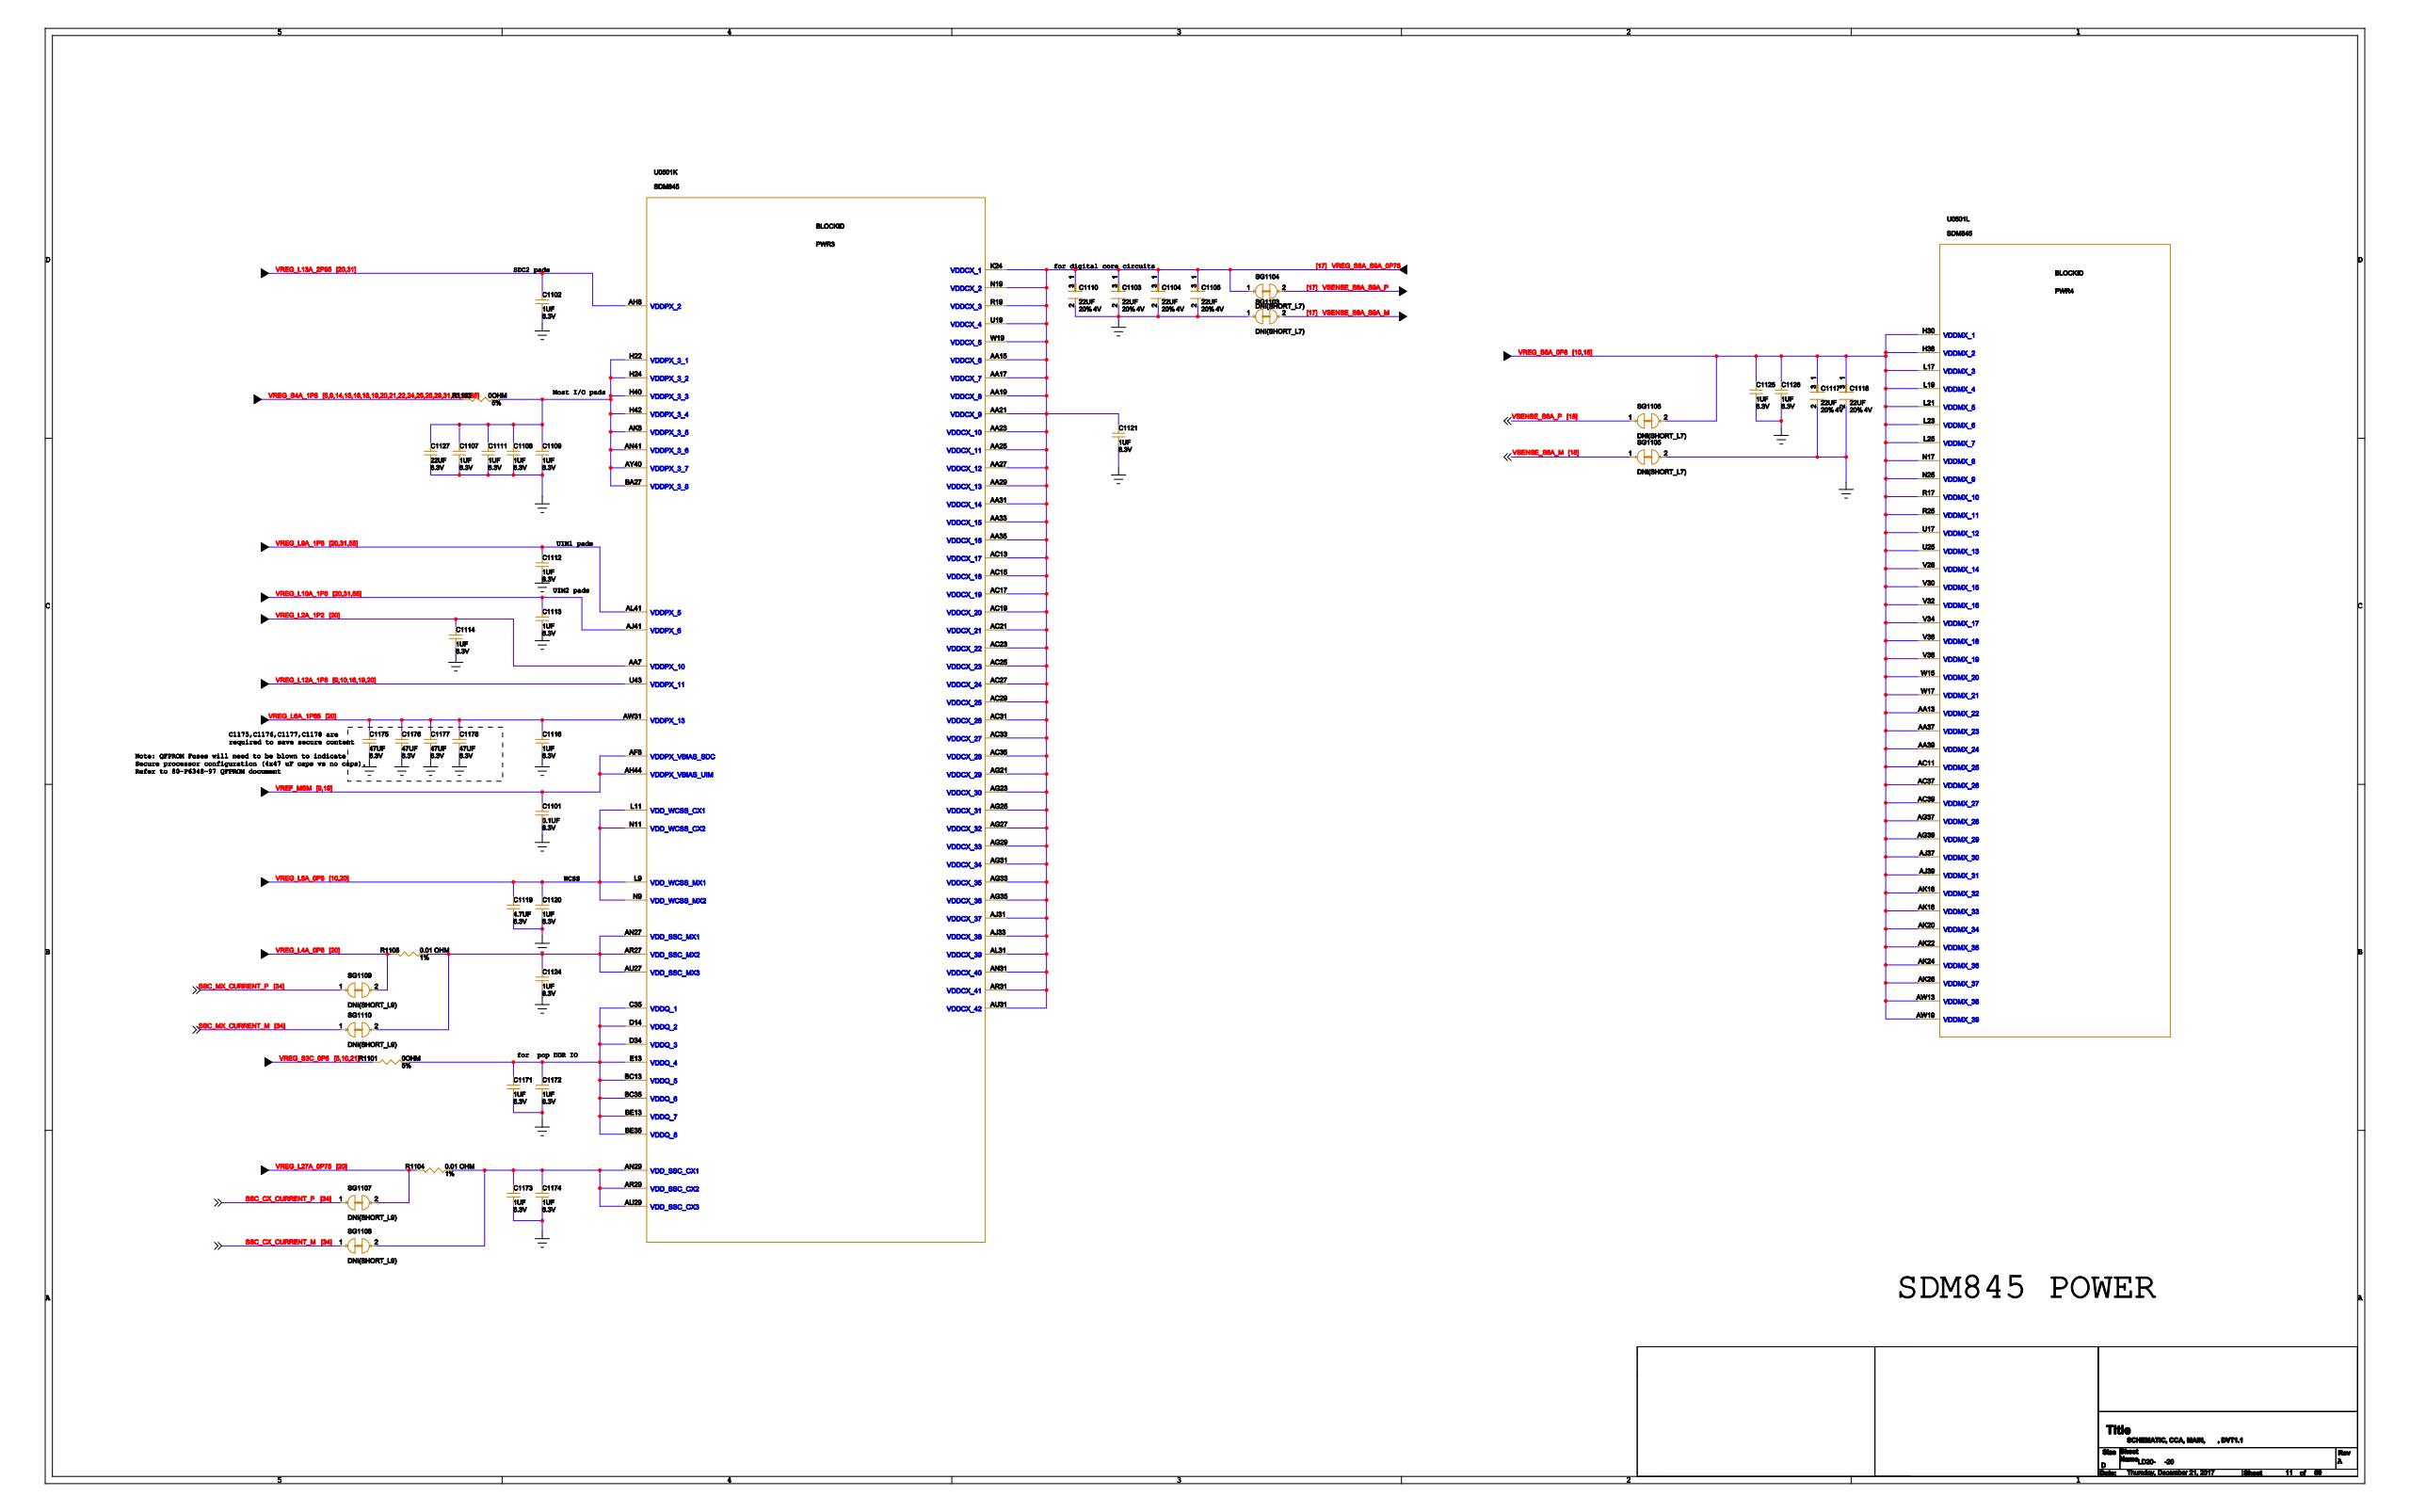Circuit board | Cadence Allegro | 1520 parts | 1149 nets | one sheet of the schematic
Parts on this sheet (reference | value | footprint):
C1101 | 0.1UF | 2P0201R
C1102 | 1UF | 2P0201R
C1103 | 22UF | 3PSM49X37N
C1104 | 22UF | 3PSM49X37N
C1105 | 22UF | 3PSM49X37N
C1107 | 1UF | 2P0201R
C1108 | 1UF | 2P0201R
C1109 | 1UF | 2P0201R
C1110 | 22UF | 3PSM49X37N
C1111 | 1UF | 2P0201R
C1112 | 1UF | 2P0201R
C1113 | 1UF | 2P0201R
C1114 | 1UF | 2P0201R
C1116 | 1UF | 2P0201R
C1117 | 22UF | 3PSM49X37N
C1118 | 22UF | 3PSM49X37N
C1119 | 4.7UF | 2P0402R
C1120 | 1UF | 2P0201R
C1121 | 1UF | 2P0201R
C1124 | 1UF | 2P0201R
C1125 | 1UF | 2P0201R
C1126 | 1UF | 2P0201R
C1127 | 22UF | 2P0603R
C1171 | 1UF | 2P0201R
C1172 | 1UF | 2P0201R
C1173 | 1UF | 2P0201R
C1174 | 1UF | 2P0201R
C1175 | 47UF | 2P0603R
C1176 | 47UF | 2P0603R
C1177 | 47UF | 2P0603R
C1178 | 47UF | 2P0603R
R1101 | 0OHM | 2P0201R
R1103 | 0OHM | 2P0201R
R1104 | 0.01 OHM | 2P0603R
R1105 | 0.01 OHM | 2P0603R
SG1103 | DNI(SHORT_L7) | SHORT_L7_2REC08X12
SG1104 | DNI(SHORT_L7) | SHORT_L7_2REC08X12
SG1105 | DNI(SHORT_L7) | SHORT_L7_2REC08X12
SG1106 | DNI(SHORT_L7) | SHORT_L7_2REC08X12
SG1107 | DNI(SHORT_L9) | SHORT_L9_2REC08X12
SG1108 | DNI(SHORT_L9) | SHORT_L9_2REC08X12
SG1109 | DNI(SHORT_L9) | SHORT_L9_2REC08X12
SG1110 | DNI(SHORT_L9) | SHORT_L9_2REC08X12
U0501 | SDM845 | 914PGA490X490B138D45
Nets of these parts (net: part-pin ...):
GND: C1101-2 C1102-2 C1103-2 C1104-2 C1105-2 C1107-2 C1108-2 C1109-2 C1110-2 C1111-2 C1112-2 C1113-2 C1114-2 C1116-2 C1117-2 C1118-2 C1119-2 C1120-2 C1121-2 C1124-2 C1125-2 C1126-2 C1127-2 C1171-2 C1172-2 C1173-2 C1174-2 C1175-2 C1176-2 C1177-2 C1178-2 SG1103-1 SG1105-2
VREG_S4A_1P8: R1103-1
SSC_CX_CURRENT_P: SG1107-1
VREG_L27A_0P75: R1104-1 SG1107-2
SSC_CX_CURRENT_M: SG1108-1
N47097967: C1173-1 C1174-1 R1104-2 SG1108-2 U0501-AN29 U0501-AR29 U0501-AU29
SSC_MX_CURRENT_P: SG1109-1
VREG_L4A_0P8: R1105-1 SG1109-2
SSC_MX_CURRENT_M: SG1110-1
N47104224: C1124-1 R1105-2 SG1110-2 U0501-AN27 U0501-AR27 U0501-AU27
VREG_S6A_0P8: C1117-1 C1117-3 C1118-1 C1118-3 C1125-1 C1126-1 SG1106-2 U0501-AA13 U0501-AA37 U0501-AA39 U0501-AC11 U0501-AC37 U0501-AC39 U0501-AG37 U0501-AG39 U0501-AJ37 U0501-AJ39 U0501-AK16 U0501-AK18 U0501-AK20 U0501-AK22 U0501-AK24 U0501-AK26 U0501-AW13 U0501-AW19 U0501-H30 U0501-H38 U0501-L17 U0501-L19 U0501-L21 U0501-L23 U0501-L25 U0501-N17 U0501-N25 U0501-R17 U0501-R25 U0501-U17 U0501-U25 U0501-V28 U0501-V30 U0501-V32 U0501-V34 U0501-V36 U0501-V38 U0501-W15 U0501-W17
VREG_S8A_S9A_0P75: C1103-1 C1103-3 C1104-1 C1104-3 C1105-1 C1105-3 C1110-1 C1110-3 C1121-1 SG1104-1 U0501-AA15 U0501-AA17 U0501-AA19 U0501-AA21 U0501-AA23 U0501-AA25 U0501-AA27 U0501-AA29 U0501-AA31 U0501-AA33 U0501-AA35 U0501-AC13 U0501-AC15 U0501-AC17 U0501-AC19 U0501-AC21 U0501-AC23 U0501-AC25 U0501-AC27 U0501-AC29 U0501-AC31 U0501-AC33 U0501-AC35 U0501-AG21 U0501-AG23 U0501-AG25 U0501-AG27 U0501-AG29 U0501-AG31 U0501-AG33 U0501-AG35 U0501-AJ31 U0501-AJ33 U0501-AL31 U0501-AN31 U0501-AR31 U0501-AU31 U0501-K24 U0501-N19 U0501-R19 U0501-U19 U0501-W19
VREG_S3C_0P6: R1101-2
VREG_L9A_1P8: C1112-1 U0501-AL41
VREG_L10A_1P8: C1113-1 U0501-AJ41
VREG_L12A_1P8: U0501-U43
VREF_MSM: C1101-1 U0501-AF8 U0501-AH44
VREG_L6A_1P85: C1116-1 C1175-1 C1176-1 C1177-1 C1178-1 U0501-AW31
VREG_L5A_0P8: C1119-1 C1120-1 U0501-L9 U0501-L11 U0501-N9 U0501-N11
VREG_L13A_2P95: C1102-1 U0501-AH8
N34049626: C1107-1 C1108-1 C1109-1 C1111-1 C1127-1 R1103-2 U0501-AK8 U0501-AN41 U0501-AY40 U0501-BA27 U0501-H22 U0501-H24 U0501-H40 U0501-H42
VREG_L2A_1P2: C1114-1 U0501-AA7
N34058949: C1171-1 C1172-1 R1101-1 U0501-BC13 U0501-BC35 U0501-BE13 U0501-BE35 U0501-C35 U0501-D14 U0501-D34 U0501-E13
VSENSE_S8A_S9A_M: SG1103-2
VSENSE_S8A_S9A_P: SG1104-2
VSENSE_S6A_M: SG1105-1
VSENSE_S6A_P: SG1106-1